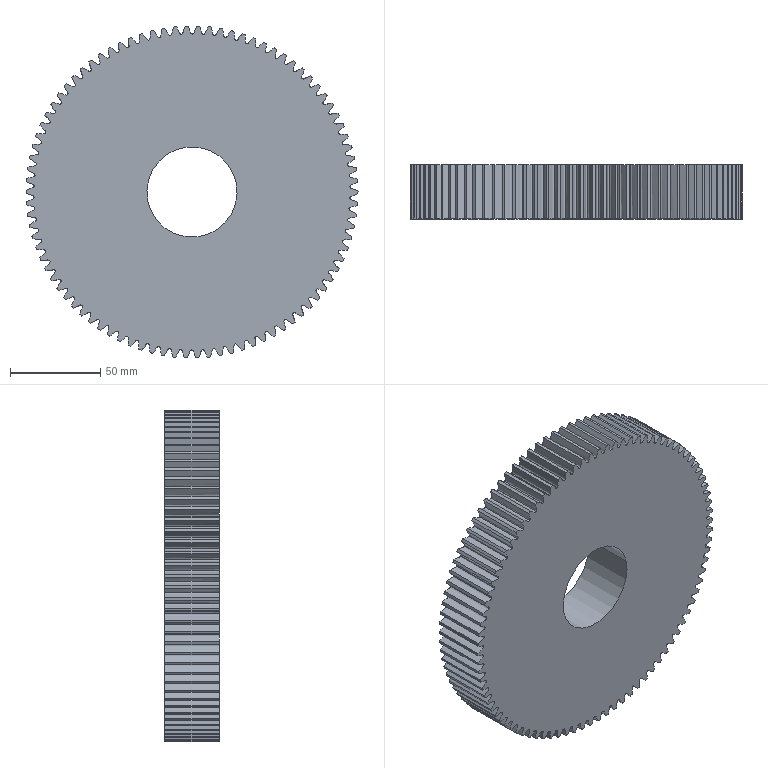Part | STEP file | 2026.6.15-Main Assembly图.sldasm-Part-50 | 1 solid | 366 faces | box 184 x 30 x 183.947 mm | volume 703550 mm3 | cylinder 184 | spline 180 | plane 2 | commonest cylinder face diameters 184 x92 174.997 x90 50 x2